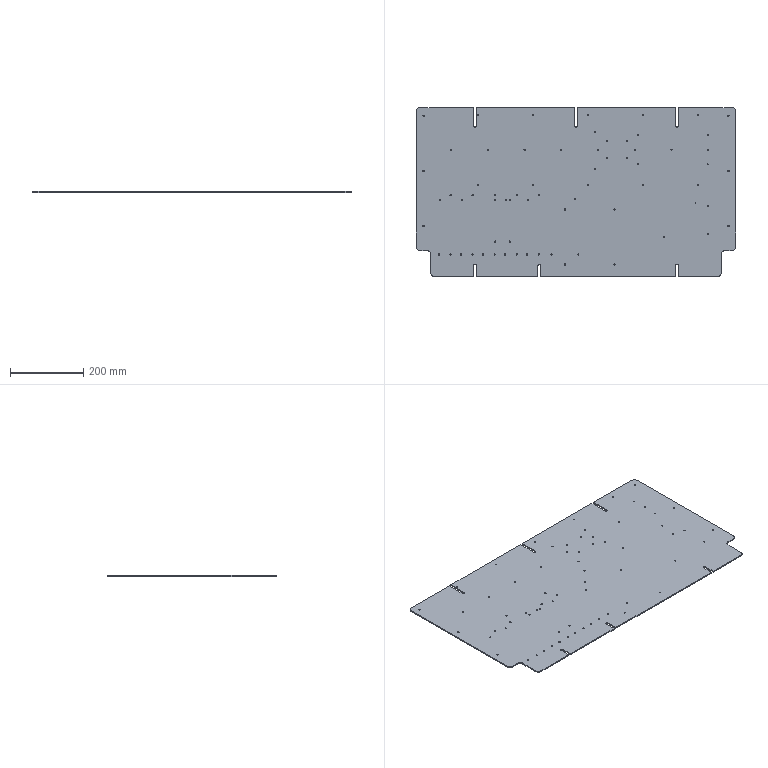Part | STEP file | 1 solid | 178 faces | box 870 x 460 x 3 mm | volume 1176521 mm3 | cylinder 150 | plane 28 | commonest cylinder face diameters 3.3 x116 2.5 x20 20 x8 7 x6